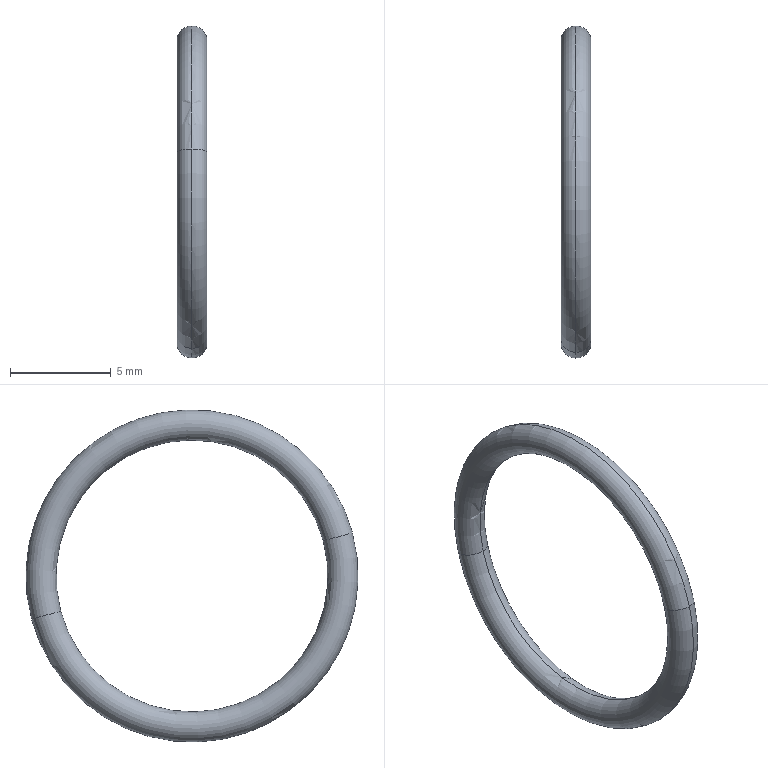Part | NX | features BREP 1 | 1 solid | 4 faces | box 1.5 x 16.5 x 16.5 mm | volume 83.275 mm3 | torus 4
STEP:
#1=CARTESIAN_POINT('',(169.717,81.783,-0.9035));
#2=VERTEX_POINT('',#1);
#3=CARTESIAN_POINT('',(169.717,68.743,2.591));
#4=VERTEX_POINT('',#3);
#5=CARTESIAN_POINT('',(169.717,75.263,0.8438));
#6=DIRECTION('',(1.,0.,0.));
#7=DIRECTION('',(0.,0.9659,-0.2589));
#8=AXIS2_PLACEMENT_3D('',#5,#6,#7);
#9=CIRCLE('',#8,6.75);
#10=EDGE_CURVE('',#2,#4,#9,.F.);
#11=ORIENTED_EDGE('',*,*,#10,.T.);
#12=CARTESIAN_POINT('',(169.717,67.294,2.979));
#13=VERTEX_POINT('',#12);
#14=CARTESIAN_POINT('',(169.717,68.018,2.785));
#15=DIRECTION('',(0.,-0.2589,-0.9659));
#16=DIRECTION('',(0.,-0.9659,0.2589));
#17=AXIS2_PLACEMENT_3D('',#14,#15,#16);
#18=CIRCLE('',#17,0.75);
#19=EDGE_CURVE('',#13,#4,#18,.F.);
#20=ORIENTED_EDGE('',*,*,#19,.F.);
#21=CARTESIAN_POINT('',(169.717,83.232,-1.292));
#22=VERTEX_POINT('',#21);
#23=CARTESIAN_POINT('',(169.717,75.263,0.8438));
#24=DIRECTION('',(1.,0.,0.));
#25=DIRECTION('',(0.,0.9659,-0.2589));
#26=AXIS2_PLACEMENT_3D('',#23,#24,#25);
#27=CIRCLE('',#26,8.25);
#28=EDGE_CURVE('',#22,#13,#27,.F.);
#29=ORIENTED_EDGE('',*,*,#28,.F.);
#30=CARTESIAN_POINT('',(169.717,82.507,-1.098));
#31=DIRECTION('',(0.,0.2589,0.9659));
#32=DIRECTION('',(0.,0.9659,-0.2589));
#33=AXIS2_PLACEMENT_3D('',#30,#31,#32);
#34=CIRCLE('',#33,0.75);
#35=EDGE_CURVE('',#22,#2,#34,.F.);
#36=ORIENTED_EDGE('',*,*,#35,.T.);
#37=EDGE_LOOP('',(#11,#20,#29,#36));
#38=FACE_BOUND('',#37,.T.);
#39=CARTESIAN_POINT('',(169.717,75.263,0.8438));
#40=DIRECTION('',(1.,0.,0.));
#41=DIRECTION('',(0.,0.,-1.));
#42=AXIS2_PLACEMENT_3D('',#39,#40,#41);
#43=TOROIDAL_SURFACE('',#42,7.5,0.75);
#44=ADVANCED_FACE('',(#38),#43,.T.);
#45=ORIENTED_EDGE('',*,*,#28,.T.);
#46=CARTESIAN_POINT('',(169.717,68.018,2.785));
#47=DIRECTION('',(0.,-0.2589,-0.9659));
#48=DIRECTION('',(0.,-0.9659,0.2589));
#49=AXIS2_PLACEMENT_3D('',#46,#47,#48);
#50=CIRCLE('',#49,0.75);
#51=EDGE_CURVE('',#4,#13,#50,.F.);
#52=ORIENTED_EDGE('',*,*,#51,.F.);
#53=ORIENTED_EDGE('',*,*,#10,.F.);
#54=CARTESIAN_POINT('',(169.717,82.507,-1.098));
#55=DIRECTION('',(0.,0.2589,0.9659));
#56=DIRECTION('',(0.,0.9659,-0.2589));
#57=AXIS2_PLACEMENT_3D('',#54,#55,#56);
#58=CIRCLE('',#57,0.75);
#59=EDGE_CURVE('',#2,#22,#58,.F.);
#60=ORIENTED_EDGE('',*,*,#59,.T.);
#61=EDGE_LOOP('',(#45,#52,#53,#60));
#62=FACE_BOUND('',#61,.T.);
#63=CARTESIAN_POINT('',(169.717,75.263,0.8438));
#64=DIRECTION('',(1.,0.,0.));
#65=DIRECTION('',(0.,0.,-1.));
#66=AXIS2_PLACEMENT_3D('',#63,#64,#65);
#67=TOROIDAL_SURFACE('',#66,7.5,0.75);
#68=ADVANCED_FACE('',(#62),#67,.T.);
#69=ORIENTED_EDGE('',*,*,#51,.T.);
#70=CARTESIAN_POINT('',(169.717,75.263,0.8438));
#71=DIRECTION('',(1.,0.,0.));
#72=DIRECTION('',(0.,0.9659,-0.2589));
#73=AXIS2_PLACEMENT_3D('',#70,#71,#72);
#74=CIRCLE('',#73,8.25);
#75=EDGE_CURVE('',#22,#13,#74,.T.);
#76=ORIENTED_EDGE('',*,*,#75,.F.);
#77=ORIENTED_EDGE('',*,*,#59,.F.);
#78=CARTESIAN_POINT('',(169.717,75.263,0.8438));
#79=DIRECTION('',(1.,0.,0.));
#80=DIRECTION('',(0.,0.9659,-0.2589));
#81=AXIS2_PLACEMENT_3D('',#78,#79,#80);
#82=CIRCLE('',#81,6.75);
#83=EDGE_CURVE('',#2,#4,#82,.T.);
#84=ORIENTED_EDGE('',*,*,#83,.T.);
#85=EDGE_LOOP('',(#69,#76,#77,#84));
#86=FACE_BOUND('',#85,.T.);
#87=CARTESIAN_POINT('',(169.717,75.263,0.8438));
#88=DIRECTION('',(1.,0.,0.));
#89=DIRECTION('',(0.,1.,0.));
#90=AXIS2_PLACEMENT_3D('',#87,#88,#89);
#91=TOROIDAL_SURFACE('',#90,7.5,0.75);
#92=ADVANCED_FACE('',(#86),#91,.T.);
#93=ORIENTED_EDGE('',*,*,#19,.T.);
#94=ORIENTED_EDGE('',*,*,#83,.F.);
#95=ORIENTED_EDGE('',*,*,#35,.F.);
#96=ORIENTED_EDGE('',*,*,#75,.T.);
#97=EDGE_LOOP('',(#93,#94,#95,#96));
#98=FACE_BOUND('',#97,.T.);
#99=CARTESIAN_POINT('',(169.717,75.263,0.8438));
#100=DIRECTION('',(1.,0.,0.));
#101=DIRECTION('',(0.,0.,-1.));
#102=AXIS2_PLACEMENT_3D('',#99,#100,#101);
#103=TOROIDAL_SURFACE('',#102,7.5,0.75);
#104=ADVANCED_FACE('',(#98),#103,.T.);
#105=CLOSED_SHELL('',(#44,#68,#92,#104));
#106=MANIFOLD_SOLID_BREP('',#105);
#107=(LENGTH_UNIT()NAMED_UNIT(*)SI_UNIT(.MILLI.,.METRE.));
#108=UNCERTAINTY_MEASURE_WITH_UNIT(LENGTH_MEASURE(0.00001),#107,'','');
#109=(NAMED_UNIT(*)PLANE_ANGLE_UNIT()SI_UNIT($,.RADIAN.));
#110=(NAMED_UNIT(*)SI_UNIT($,.STERADIAN.)SOLID_ANGLE_UNIT());
#111=(GEOMETRIC_REPRESENTATION_CONTEXT(3)GLOBAL_UNCERTAINTY_ASSIGNED_CONTEXT((#108))GLOBAL_UNIT_ASSIGNED_CONTEXT((#107,#109,#110))REPRESENTATION_CONTEXT('',''));
#112=ADVANCED_BREP_SHAPE_REPRESENTATION('',(#106),#111);